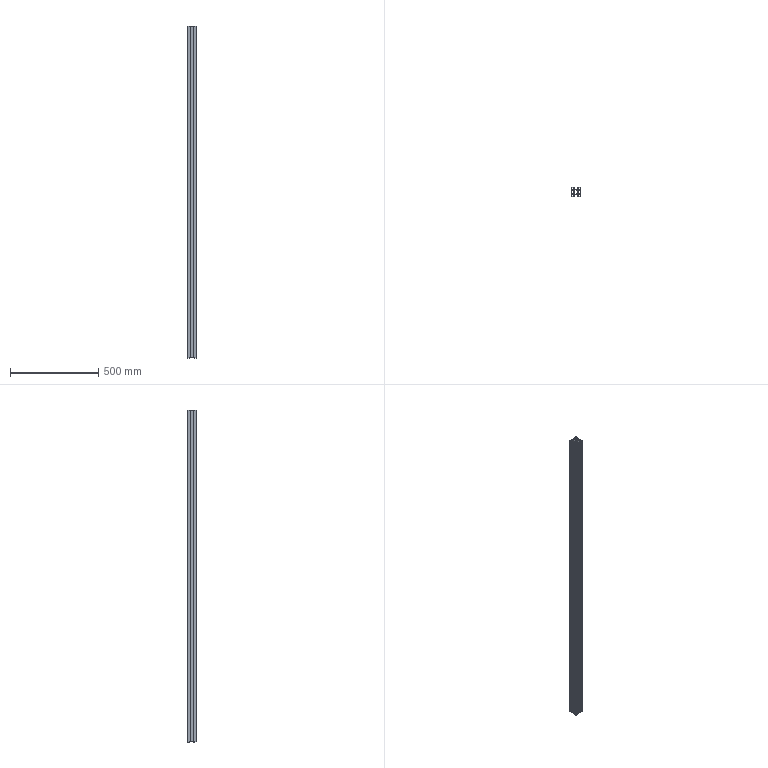Part | STEP file | 46A-00006CC11-1880mm | 1 solid | 142 faces | box 50 x 50 x 1880 mm | volume 1104486 mm3 | cylinder 84 | plane 58 | commonest cylinder face diameters 1 x24 4 x24 1.5 x16 3.7 x8 6.7 x8 2 x4